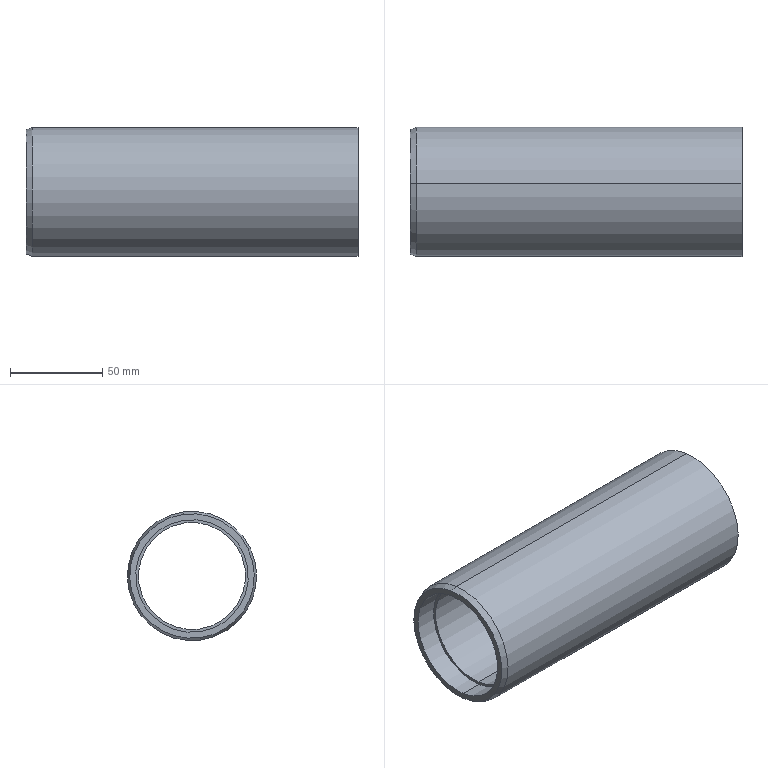Part | NX | features BREP 1 | 1 solid | 11 faces | box 179.9 x 70 x 70 mm | volume 213177 mm3 | cylinder 6 | plane 3 | cone 2 | commonest cylinder face diameters 58 x2 61 x2 70 x2
STEP:
#1=CARTESIAN_POINT('',(-530.465,4.551,33.418));
#2=VERTEX_POINT('',#1);
#3=CARTESIAN_POINT('',(-530.465,-4.551,-33.418));
#4=VERTEX_POINT('',#3);
#5=CARTESIAN_POINT('',(-530.465,0.,0.));
#6=DIRECTION('',(-1.,0.,0.));
#7=DIRECTION('',(0.,-0.1349,-0.9909));
#8=AXIS2_PLACEMENT_3D('',#5,#6,#7);
#9=CIRCLE('',#8,33.726);
#10=EDGE_CURVE('',#2,#4,#9,.T.);
#11=ORIENTED_EDGE('',*,*,#10,.F.);
#12=CARTESIAN_POINT('',(-526.965,4.722,34.68));
#13=VERTEX_POINT('',#12);
#14=CARTESIAN_POINT('',(-530.465,4.551,33.418));
#15=DIRECTION('',(0.9397,0.04615,0.3389));
#16=VECTOR('',#15,1000.);
#17=LINE('',#14,#16);
#18=EDGE_CURVE('',#13,#2,#17,.F.);
#19=ORIENTED_EDGE('',*,*,#18,.F.);
#20=CARTESIAN_POINT('',(-526.965,-4.722,-34.68));
#21=VERTEX_POINT('',#20);
#22=CARTESIAN_POINT('',(-526.965,0.,0.));
#23=DIRECTION('',(1.,0.,0.));
#24=DIRECTION('',(0.,-0.1349,-0.9909));
#25=AXIS2_PLACEMENT_3D('',#22,#23,#24);
#26=CIRCLE('',#25,35.);
#27=EDGE_CURVE('',#21,#13,#26,.T.);
#28=ORIENTED_EDGE('',*,*,#27,.F.);
#29=CARTESIAN_POINT('',(-530.465,-4.551,-33.418));
#30=DIRECTION('',(0.9397,-0.04615,-0.3389));
#31=VECTOR('',#30,1000.);
#32=LINE('',#29,#31);
#33=EDGE_CURVE('',#21,#4,#32,.F.);
#34=ORIENTED_EDGE('',*,*,#33,.T.);
#35=EDGE_LOOP('',(#11,#19,#28,#34));
#36=FACE_BOUND('',#35,.T.);
#37=CARTESIAN_POINT('',(-530.465,0.,0.));
#38=DIRECTION('',(1.,0.,0.));
#39=DIRECTION('',(0.,0.1349,0.9909));
#40=AXIS2_PLACEMENT_3D('',#37,#38,#39);
#41=CONICAL_SURFACE('',#40,33.726,0.3491);
#42=ADVANCED_FACE('',(#36),#41,.T.);
#43=CARTESIAN_POINT('',(-518.465,-4.115,-30.221));
#44=VERTEX_POINT('',#43);
#45=CARTESIAN_POINT('',(-518.465,4.115,30.221));
#46=VERTEX_POINT('',#45);
#47=CARTESIAN_POINT('',(-518.465,0.,0.));
#48=DIRECTION('',(-1.,0.,0.));
#49=DIRECTION('',(0.,0.1349,0.9909));
#50=AXIS2_PLACEMENT_3D('',#47,#48,#49);
#51=CIRCLE('',#50,30.5);
#52=EDGE_CURVE('',#44,#46,#51,.T.);
#53=ORIENTED_EDGE('',*,*,#52,.F.);
#54=CARTESIAN_POINT('',(-530.465,-4.115,-30.221));
#55=VERTEX_POINT('',#54);
#56=CARTESIAN_POINT('',(-530.465,-4.115,-30.221));
#57=DIRECTION('',(-1.,0.,0.));
#58=VECTOR('',#57,1000.);
#59=LINE('',#56,#58);
#60=EDGE_CURVE('',#44,#55,#59,.T.);
#61=ORIENTED_EDGE('',*,*,#60,.T.);
#62=CARTESIAN_POINT('',(-530.465,4.115,30.221));
#63=VERTEX_POINT('',#62);
#64=CARTESIAN_POINT('',(-530.465,0.,0.));
#65=DIRECTION('',(-1.,0.,0.));
#66=DIRECTION('',(0.,0.1349,0.9909));
#67=AXIS2_PLACEMENT_3D('',#64,#65,#66);
#68=CIRCLE('',#67,30.5);
#69=EDGE_CURVE('',#55,#63,#68,.T.);
#70=ORIENTED_EDGE('',*,*,#69,.T.);
#71=CARTESIAN_POINT('',(-530.465,4.115,30.221));
#72=DIRECTION('',(-1.,0.,0.));
#73=VECTOR('',#72,1000.);
#74=LINE('',#71,#73);
#75=EDGE_CURVE('',#46,#63,#74,.T.);
#76=ORIENTED_EDGE('',*,*,#75,.F.);
#77=EDGE_LOOP('',(#53,#61,#70,#76));
#78=FACE_BOUND('',#77,.T.);
#79=CARTESIAN_POINT('',(-530.465,0.,0.));
#80=DIRECTION('',(-1.,0.,0.));
#81=DIRECTION('',(0.,-0.1349,-0.9909));
#82=AXIS2_PLACEMENT_3D('',#79,#80,#81);
#83=CYLINDRICAL_SURFACE('',#82,30.5);
#84=ADVANCED_FACE('',(#78),#83,.F.);
#85=CARTESIAN_POINT('',(-350.565,3.913,28.735));
#86=VERTEX_POINT('',#85);
#87=CARTESIAN_POINT('',(-350.565,-3.913,-28.735));
#88=VERTEX_POINT('',#87);
#89=CARTESIAN_POINT('',(-350.565,0.,0.));
#90=DIRECTION('',(1.,0.,0.));
#91=DIRECTION('',(0.,0.,1.));
#92=AXIS2_PLACEMENT_3D('',#89,#90,#91);
#93=CIRCLE('',#92,29.);
#94=EDGE_CURVE('',#86,#88,#93,.T.);
#95=ORIENTED_EDGE('',*,*,#94,.T.);
#96=CARTESIAN_POINT('',(-518.465,-3.913,-28.735));
#97=VERTEX_POINT('',#96);
#98=CARTESIAN_POINT('',(-530.465,-3.913,-28.735));
#99=DIRECTION('',(-1.,0.,0.));
#100=VECTOR('',#99,1000.);
#101=LINE('',#98,#100);
#102=EDGE_CURVE('',#88,#97,#101,.T.);
#103=ORIENTED_EDGE('',*,*,#102,.T.);
#104=CARTESIAN_POINT('',(-518.465,3.913,28.735));
#105=VERTEX_POINT('',#104);
#106=CARTESIAN_POINT('',(-518.465,0.,0.));
#107=DIRECTION('',(-1.,0.,0.));
#108=DIRECTION('',(0.,0.1349,0.9909));
#109=AXIS2_PLACEMENT_3D('',#106,#107,#108);
#110=CIRCLE('',#109,29.);
#111=EDGE_CURVE('',#97,#105,#110,.T.);
#112=ORIENTED_EDGE('',*,*,#111,.T.);
#113=CARTESIAN_POINT('',(-530.465,3.913,28.735));
#114=DIRECTION('',(-1.,0.,0.));
#115=VECTOR('',#114,1000.);
#116=LINE('',#113,#115);
#117=EDGE_CURVE('',#86,#105,#116,.T.);
#118=ORIENTED_EDGE('',*,*,#117,.F.);
#119=EDGE_LOOP('',(#95,#103,#112,#118));
#120=FACE_BOUND('',#119,.T.);
#121=CARTESIAN_POINT('',(-530.465,0.,0.));
#122=DIRECTION('',(-1.,0.,0.));
#123=DIRECTION('',(0.,-0.1349,-0.9909));
#124=AXIS2_PLACEMENT_3D('',#121,#122,#123);
#125=CYLINDRICAL_SURFACE('',#124,29.);
#126=ADVANCED_FACE('',(#120),#125,.F.);
#127=CARTESIAN_POINT('',(-350.565,4.722,34.68));
#128=VERTEX_POINT('',#127);
#129=CARTESIAN_POINT('',(-350.565,-4.722,-34.68));
#130=VERTEX_POINT('',#129);
#131=CARTESIAN_POINT('',(-350.565,0.,0.));
#132=DIRECTION('',(-1.,0.,0.));
#133=DIRECTION('',(0.,0.,1.));
#134=AXIS2_PLACEMENT_3D('',#131,#132,#133);
#135=CIRCLE('',#134,35.);
#136=EDGE_CURVE('',#128,#130,#135,.T.);
#137=ORIENTED_EDGE('',*,*,#136,.T.);
#138=CARTESIAN_POINT('',(-530.465,-4.722,-34.68));
#139=DIRECTION('',(-1.,0.,0.));
#140=VECTOR('',#139,1000.);
#141=LINE('',#138,#140);
#142=EDGE_CURVE('',#130,#21,#141,.T.);
#143=ORIENTED_EDGE('',*,*,#142,.T.);
#144=ORIENTED_EDGE('',*,*,#27,.T.);
#145=CARTESIAN_POINT('',(-530.465,4.722,34.68));
#146=DIRECTION('',(-1.,0.,0.));
#147=VECTOR('',#146,1000.);
#148=LINE('',#145,#147);
#149=EDGE_CURVE('',#128,#13,#148,.T.);
#150=ORIENTED_EDGE('',*,*,#149,.F.);
#151=EDGE_LOOP('',(#137,#143,#144,#150));
#152=FACE_BOUND('',#151,.T.);
#153=CARTESIAN_POINT('',(-530.465,0.,0.));
#154=DIRECTION('',(-1.,0.,0.));
#155=DIRECTION('',(0.,-0.1349,-0.9909));
#156=AXIS2_PLACEMENT_3D('',#153,#154,#155);
#157=CYLINDRICAL_SURFACE('',#156,35.);
#158=ADVANCED_FACE('',(#152),#157,.T.);
#159=ORIENTED_EDGE('',*,*,#142,.F.);
#160=CARTESIAN_POINT('',(-350.565,0.,0.));
#161=DIRECTION('',(-1.,0.,0.));
#162=DIRECTION('',(0.,0.,1.));
#163=AXIS2_PLACEMENT_3D('',#160,#161,#162);
#164=CIRCLE('',#163,35.);
#165=EDGE_CURVE('',#130,#128,#164,.T.);
#166=ORIENTED_EDGE('',*,*,#165,.T.);
#167=ORIENTED_EDGE('',*,*,#149,.T.);
#168=CARTESIAN_POINT('',(-526.965,0.,0.));
#169=DIRECTION('',(1.,0.,0.));
#170=DIRECTION('',(0.,-0.1349,-0.9909));
#171=AXIS2_PLACEMENT_3D('',#168,#169,#170);
#172=CIRCLE('',#171,35.);
#173=EDGE_CURVE('',#13,#21,#172,.T.);
#174=ORIENTED_EDGE('',*,*,#173,.T.);
#175=EDGE_LOOP('',(#159,#166,#167,#174));
#176=FACE_BOUND('',#175,.T.);
#177=CARTESIAN_POINT('',(-530.465,0.,0.));
#178=DIRECTION('',(-1.,0.,0.));
#179=DIRECTION('',(0.,-0.1349,-0.9909));
#180=AXIS2_PLACEMENT_3D('',#177,#178,#179);
#181=CYLINDRICAL_SURFACE('',#180,35.);
#182=ADVANCED_FACE('',(#176),#181,.T.);
#183=CARTESIAN_POINT('',(-530.465,0.,0.));
#184=DIRECTION('',(-1.,0.,0.));
#185=DIRECTION('',(0.,-0.1349,-0.9909));
#186=AXIS2_PLACEMENT_3D('',#183,#184,#185);
#187=CIRCLE('',#186,33.726);
#188=EDGE_CURVE('',#4,#2,#187,.T.);
#189=ORIENTED_EDGE('',*,*,#188,.T.);
#190=ORIENTED_EDGE('',*,*,#10,.T.);
#191=EDGE_LOOP('',(#189,#190));
#192=FACE_BOUND('',#191,.T.);
#193=CARTESIAN_POINT('',(-530.465,0.,0.));
#194=DIRECTION('',(-1.,0.,0.));
#195=DIRECTION('',(0.,0.1349,0.9909));
#196=AXIS2_PLACEMENT_3D('',#193,#194,#195);
#197=CIRCLE('',#196,30.5);
#198=EDGE_CURVE('',#63,#55,#197,.T.);
#199=ORIENTED_EDGE('',*,*,#198,.F.);
#200=ORIENTED_EDGE('',*,*,#69,.F.);
#201=EDGE_LOOP('',(#199,#200));
#202=FACE_BOUND('',#201,.T.);
#203=CARTESIAN_POINT('',(-530.465,34.68,-4.722));
#204=DIRECTION('',(1.,0.,0.));
#205=DIRECTION('',(0.,0.1349,0.9909));
#206=AXIS2_PLACEMENT_3D('',#203,#204,#205);
#207=PLANE('',#206);
#208=ADVANCED_FACE('',(#192,#202),#207,.F.);
#209=ORIENTED_EDGE('',*,*,#102,.F.);
#210=CARTESIAN_POINT('',(-350.565,0.,0.));
#211=DIRECTION('',(1.,0.,0.));
#212=DIRECTION('',(0.,0.,1.));
#213=AXIS2_PLACEMENT_3D('',#210,#211,#212);
#214=CIRCLE('',#213,29.);
#215=EDGE_CURVE('',#88,#86,#214,.T.);
#216=ORIENTED_EDGE('',*,*,#215,.T.);
#217=ORIENTED_EDGE('',*,*,#117,.T.);
#218=CARTESIAN_POINT('',(-518.465,0.,0.));
#219=DIRECTION('',(-1.,0.,0.));
#220=DIRECTION('',(0.,0.1349,0.9909));
#221=AXIS2_PLACEMENT_3D('',#218,#219,#220);
#222=CIRCLE('',#221,29.);
#223=EDGE_CURVE('',#105,#97,#222,.T.);
#224=ORIENTED_EDGE('',*,*,#223,.T.);
#225=EDGE_LOOP('',(#209,#216,#217,#224));
#226=FACE_BOUND('',#225,.T.);
#227=CARTESIAN_POINT('',(-530.465,0.,0.));
#228=DIRECTION('',(-1.,0.,0.));
#229=DIRECTION('',(0.,-0.1349,-0.9909));
#230=AXIS2_PLACEMENT_3D('',#227,#228,#229);
#231=CYLINDRICAL_SURFACE('',#230,29.);
#232=ADVANCED_FACE('',(#226),#231,.F.);
#233=ORIENTED_EDGE('',*,*,#223,.F.);
#234=ORIENTED_EDGE('',*,*,#111,.F.);
#235=EDGE_LOOP('',(#233,#234));
#236=FACE_BOUND('',#235,.T.);
#237=CARTESIAN_POINT('',(-518.465,0.,0.));
#238=DIRECTION('',(-1.,0.,0.));
#239=DIRECTION('',(0.,0.1349,0.9909));
#240=AXIS2_PLACEMENT_3D('',#237,#238,#239);
#241=CIRCLE('',#240,30.5);
#242=EDGE_CURVE('',#46,#44,#241,.T.);
#243=ORIENTED_EDGE('',*,*,#242,.T.);
#244=ORIENTED_EDGE('',*,*,#52,.T.);
#245=EDGE_LOOP('',(#243,#244));
#246=FACE_BOUND('',#245,.T.);
#247=CARTESIAN_POINT('',(-518.465,28.735,-3.913));
#248=DIRECTION('',(1.,0.,0.));
#249=DIRECTION('',(0.,0.1349,0.9909));
#250=AXIS2_PLACEMENT_3D('',#247,#248,#249);
#251=PLANE('',#250);
#252=ADVANCED_FACE('',(#236,#246),#251,.F.);
#253=ORIENTED_EDGE('',*,*,#60,.F.);
#254=ORIENTED_EDGE('',*,*,#242,.F.);
#255=ORIENTED_EDGE('',*,*,#75,.T.);
#256=ORIENTED_EDGE('',*,*,#198,.T.);
#257=EDGE_LOOP('',(#253,#254,#255,#256));
#258=FACE_BOUND('',#257,.T.);
#259=CARTESIAN_POINT('',(-530.465,0.,0.));
#260=DIRECTION('',(-1.,0.,0.));
#261=DIRECTION('',(0.,-0.1349,-0.9909));
#262=AXIS2_PLACEMENT_3D('',#259,#260,#261);
#263=CYLINDRICAL_SURFACE('',#262,30.5);
#264=ADVANCED_FACE('',(#258),#263,.F.);
#265=ORIENTED_EDGE('',*,*,#18,.T.);
#266=ORIENTED_EDGE('',*,*,#188,.F.);
#267=ORIENTED_EDGE('',*,*,#33,.F.);
#268=ORIENTED_EDGE('',*,*,#173,.F.);
#269=EDGE_LOOP('',(#265,#266,#267,#268));
#270=FACE_BOUND('',#269,.T.);
#271=CARTESIAN_POINT('',(-530.465,0.,0.));
#272=DIRECTION('',(1.,0.,0.));
#273=DIRECTION('',(0.,0.1349,0.9909));
#274=AXIS2_PLACEMENT_3D('',#271,#272,#273);
#275=CONICAL_SURFACE('',#274,33.726,0.3491);
#276=ADVANCED_FACE('',(#270),#275,.T.);
#277=ORIENTED_EDGE('',*,*,#94,.F.);
#278=ORIENTED_EDGE('',*,*,#215,.F.);
#279=EDGE_LOOP('',(#277,#278));
#280=FACE_BOUND('',#279,.T.);
#281=ORIENTED_EDGE('',*,*,#136,.F.);
#282=ORIENTED_EDGE('',*,*,#165,.F.);
#283=EDGE_LOOP('',(#281,#282));
#284=FACE_BOUND('',#283,.T.);
#285=CARTESIAN_POINT('',(-350.565,0.,0.));
#286=DIRECTION('',(-1.,0.,0.));
#287=DIRECTION('',(0.,0.,-1.));
#288=AXIS2_PLACEMENT_3D('',#285,#286,#287);
#289=PLANE('',#288);
#290=ADVANCED_FACE('',(#280,#284),#289,.F.);
#291=CLOSED_SHELL('',(#42,#84,#126,#158,#182,#208,#232,#252,#264,#276,#290));
#292=MANIFOLD_SOLID_BREP('',#291);
#293=(LENGTH_UNIT()NAMED_UNIT(*)SI_UNIT(.MILLI.,.METRE.));
#294=UNCERTAINTY_MEASURE_WITH_UNIT(LENGTH_MEASURE(0.00001),#293,'','');
#295=(NAMED_UNIT(*)PLANE_ANGLE_UNIT()SI_UNIT($,.RADIAN.));
#296=(NAMED_UNIT(*)SI_UNIT($,.STERADIAN.)SOLID_ANGLE_UNIT());
#297=(GEOMETRIC_REPRESENTATION_CONTEXT(3)GLOBAL_UNCERTAINTY_ASSIGNED_CONTEXT((#294))GLOBAL_UNIT_ASSIGNED_CONTEXT((#293,#295,#296))REPRESENTATION_CONTEXT('',''));
#298=ADVANCED_BREP_SHAPE_REPRESENTATION('',(#292),#297);